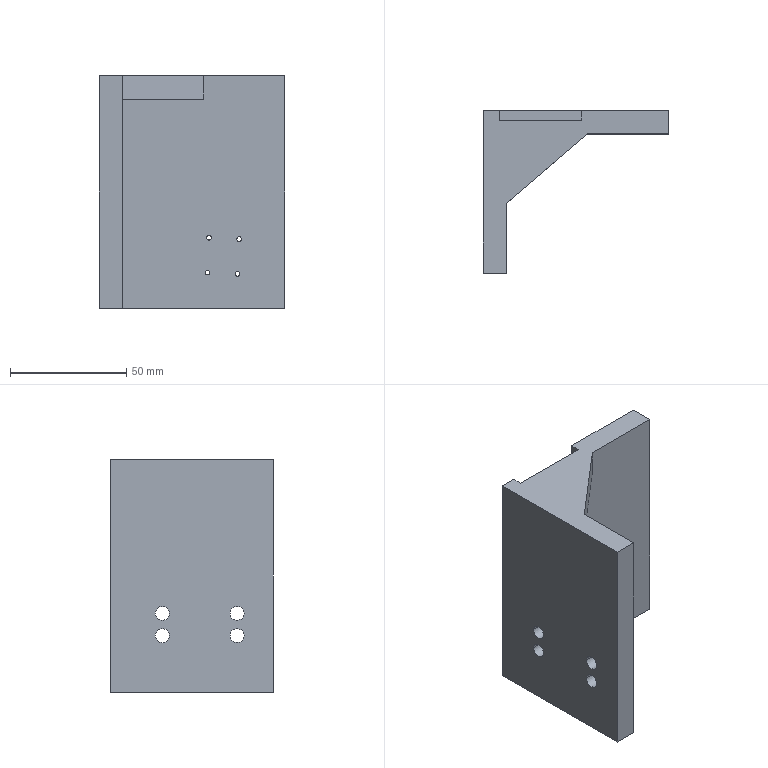Part | SolidWorks | features Cut 3, Extrusion 1, Rib 1 | 1 solid | 30 faces | box 80 x 70 x 100 mm | volume 135093 mm3 | cylinder 16 | plane 14 | commonest cylinder face diameters 2 x8 6 x8
STEP:
#1=CARTESIAN_POINT('',(8.816,32.788,30.301));
#2=VERTEX_POINT('',#1);
#3=CARTESIAN_POINT('',(10.816,32.788,30.301));
#4=VERTEX_POINT('',#3);
#5=CARTESIAN_POINT('',(9.816,32.788,30.301));
#6=DIRECTION('',(0.,-1.,0.));
#7=DIRECTION('',(1.,0.,0.));
#8=AXIS2_PLACEMENT_3D('',#5,#6,#7);
#9=CIRCLE('',#8,1.);
#10=EDGE_CURVE('',#2,#4,#9,.T.);
#11=ORIENTED_EDGE('',*,*,#10,.F.);
#12=CARTESIAN_POINT('',(8.816,22.788,30.301));
#13=VERTEX_POINT('',#12);
#14=CARTESIAN_POINT('',(8.816,37.788,30.301));
#15=DIRECTION('',(0.,-1.,0.));
#16=VECTOR('',#15,1000.);
#17=LINE('',#14,#16);
#18=EDGE_CURVE('',#2,#13,#17,.T.);
#19=ORIENTED_EDGE('',*,*,#18,.T.);
#20=CARTESIAN_POINT('',(10.816,22.788,30.301));
#21=VERTEX_POINT('',#20);
#22=CARTESIAN_POINT('',(9.816,22.788,30.301));
#23=DIRECTION('',(0.,-1.,0.));
#24=DIRECTION('',(1.,0.,0.));
#25=AXIS2_PLACEMENT_3D('',#22,#23,#24);
#26=CIRCLE('',#25,1.);
#27=EDGE_CURVE('',#13,#21,#26,.T.);
#28=ORIENTED_EDGE('',*,*,#27,.T.);
#29=CARTESIAN_POINT('',(10.816,37.788,30.301));
#30=DIRECTION('',(0.,-1.,0.));
#31=VECTOR('',#30,1000.);
#32=LINE('',#29,#31);
#33=EDGE_CURVE('',#4,#21,#32,.T.);
#34=ORIENTED_EDGE('',*,*,#33,.F.);
#35=EDGE_LOOP('',(#11,#19,#28,#34));
#36=FACE_OUTER_BOUND('',#35,.T.);
#37=CARTESIAN_POINT('',(9.816,37.788,30.301));
#38=DIRECTION('',(0.,-1.,0.));
#39=DIRECTION('',(1.,0.,0.));
#40=AXIS2_PLACEMENT_3D('',#37,#38,#39);
#41=CYLINDRICAL_SURFACE('',#40,1.);
#42=ADVANCED_FACE('',(#36),#41,.F.);
#43=CARTESIAN_POINT('',(21.15,32.788,14.748));
#44=VERTEX_POINT('',#43);
#45=CARTESIAN_POINT('',(23.15,32.788,14.748));
#46=VERTEX_POINT('',#45);
#47=CARTESIAN_POINT('',(22.15,32.788,14.748));
#48=DIRECTION('',(0.,-1.,0.));
#49=DIRECTION('',(1.,0.,0.));
#50=AXIS2_PLACEMENT_3D('',#47,#48,#49);
#51=CIRCLE('',#50,1.);
#52=EDGE_CURVE('',#44,#46,#51,.T.);
#53=ORIENTED_EDGE('',*,*,#52,.F.);
#54=CARTESIAN_POINT('',(21.15,22.788,14.748));
#55=VERTEX_POINT('',#54);
#56=CARTESIAN_POINT('',(21.15,37.788,14.748));
#57=DIRECTION('',(0.,-1.,0.));
#58=VECTOR('',#57,1000.);
#59=LINE('',#56,#58);
#60=EDGE_CURVE('',#44,#55,#59,.T.);
#61=ORIENTED_EDGE('',*,*,#60,.T.);
#62=CARTESIAN_POINT('',(23.15,22.788,14.748));
#63=VERTEX_POINT('',#62);
#64=CARTESIAN_POINT('',(22.15,22.788,14.748));
#65=DIRECTION('',(0.,-1.,0.));
#66=DIRECTION('',(1.,0.,0.));
#67=AXIS2_PLACEMENT_3D('',#64,#65,#66);
#68=CIRCLE('',#67,1.);
#69=EDGE_CURVE('',#55,#63,#68,.T.);
#70=ORIENTED_EDGE('',*,*,#69,.T.);
#71=CARTESIAN_POINT('',(23.15,37.788,14.748));
#72=DIRECTION('',(0.,-1.,0.));
#73=VECTOR('',#72,1000.);
#74=LINE('',#71,#73);
#75=EDGE_CURVE('',#46,#63,#74,.T.);
#76=ORIENTED_EDGE('',*,*,#75,.F.);
#77=EDGE_LOOP('',(#53,#61,#70,#76));
#78=FACE_OUTER_BOUND('',#77,.T.);
#79=CARTESIAN_POINT('',(22.15,37.788,14.748));
#80=DIRECTION('',(0.,-1.,0.));
#81=DIRECTION('',(1.,0.,0.));
#82=AXIS2_PLACEMENT_3D('',#79,#80,#81);
#83=CYLINDRICAL_SURFACE('',#82,1.);
#84=ADVANCED_FACE('',(#78),#83,.F.);
#85=CARTESIAN_POINT('',(21.804,32.788,29.734));
#86=VERTEX_POINT('',#85);
#87=CARTESIAN_POINT('',(23.804,32.788,29.734));
#88=VERTEX_POINT('',#87);
#89=CARTESIAN_POINT('',(22.804,32.788,29.734));
#90=DIRECTION('',(0.,-1.,0.));
#91=DIRECTION('',(1.,0.,0.));
#92=AXIS2_PLACEMENT_3D('',#89,#90,#91);
#93=CIRCLE('',#92,1.);
#94=EDGE_CURVE('',#86,#88,#93,.T.);
#95=ORIENTED_EDGE('',*,*,#94,.F.);
#96=CARTESIAN_POINT('',(21.804,22.788,29.734));
#97=VERTEX_POINT('',#96);
#98=CARTESIAN_POINT('',(21.804,37.788,29.734));
#99=DIRECTION('',(0.,-1.,0.));
#100=VECTOR('',#99,1000.);
#101=LINE('',#98,#100);
#102=EDGE_CURVE('',#86,#97,#101,.T.);
#103=ORIENTED_EDGE('',*,*,#102,.T.);
#104=CARTESIAN_POINT('',(23.804,22.788,29.734));
#105=VERTEX_POINT('',#104);
#106=CARTESIAN_POINT('',(22.804,22.788,29.734));
#107=DIRECTION('',(0.,-1.,0.));
#108=DIRECTION('',(1.,0.,0.));
#109=AXIS2_PLACEMENT_3D('',#106,#107,#108);
#110=CIRCLE('',#109,1.);
#111=EDGE_CURVE('',#97,#105,#110,.T.);
#112=ORIENTED_EDGE('',*,*,#111,.T.);
#113=CARTESIAN_POINT('',(23.804,37.788,29.734));
#114=DIRECTION('',(0.,-1.,0.));
#115=VECTOR('',#114,1000.);
#116=LINE('',#113,#115);
#117=EDGE_CURVE('',#88,#105,#116,.T.);
#118=ORIENTED_EDGE('',*,*,#117,.F.);
#119=EDGE_LOOP('',(#95,#103,#112,#118));
#120=FACE_OUTER_BOUND('',#119,.T.);
#121=CARTESIAN_POINT('',(22.804,37.788,29.734));
#122=DIRECTION('',(0.,-1.,0.));
#123=DIRECTION('',(1.,0.,0.));
#124=AXIS2_PLACEMENT_3D('',#121,#122,#123);
#125=CYLINDRICAL_SURFACE('',#124,1.);
#126=ADVANCED_FACE('',(#120),#125,.F.);
#127=CARTESIAN_POINT('',(8.162,32.788,15.315));
#128=VERTEX_POINT('',#127);
#129=CARTESIAN_POINT('',(10.162,32.788,15.315));
#130=VERTEX_POINT('',#129);
#131=CARTESIAN_POINT('',(9.162,32.788,15.315));
#132=DIRECTION('',(0.,-1.,0.));
#133=DIRECTION('',(1.,0.,0.));
#134=AXIS2_PLACEMENT_3D('',#131,#132,#133);
#135=CIRCLE('',#134,1.);
#136=EDGE_CURVE('',#128,#130,#135,.T.);
#137=ORIENTED_EDGE('',*,*,#136,.F.);
#138=CARTESIAN_POINT('',(8.162,22.788,15.315));
#139=VERTEX_POINT('',#138);
#140=CARTESIAN_POINT('',(8.162,37.788,15.315));
#141=DIRECTION('',(0.,-1.,0.));
#142=VECTOR('',#141,1000.);
#143=LINE('',#140,#142);
#144=EDGE_CURVE('',#128,#139,#143,.T.);
#145=ORIENTED_EDGE('',*,*,#144,.T.);
#146=CARTESIAN_POINT('',(10.162,22.788,15.315));
#147=VERTEX_POINT('',#146);
#148=CARTESIAN_POINT('',(9.162,22.788,15.315));
#149=DIRECTION('',(0.,-1.,0.));
#150=DIRECTION('',(1.,0.,0.));
#151=AXIS2_PLACEMENT_3D('',#148,#149,#150);
#152=CIRCLE('',#151,1.);
#153=EDGE_CURVE('',#139,#147,#152,.T.);
#154=ORIENTED_EDGE('',*,*,#153,.T.);
#155=CARTESIAN_POINT('',(10.162,37.788,15.315));
#156=DIRECTION('',(0.,-1.,0.));
#157=VECTOR('',#156,1000.);
#158=LINE('',#155,#157);
#159=EDGE_CURVE('',#130,#147,#158,.T.);
#160=ORIENTED_EDGE('',*,*,#159,.F.);
#161=EDGE_LOOP('',(#137,#145,#154,#160));
#162=FACE_OUTER_BOUND('',#161,.T.);
#163=CARTESIAN_POINT('',(9.162,37.788,15.315));
#164=DIRECTION('',(0.,-1.,0.));
#165=DIRECTION('',(1.,0.,0.));
#166=AXIS2_PLACEMENT_3D('',#163,#164,#165);
#167=CYLINDRICAL_SURFACE('',#166,1.);
#168=ADVANCED_FACE('',(#162),#167,.F.);
#169=CARTESIAN_POINT('',(-37.5,-18.605,24.355));
#170=VERTEX_POINT('',#169);
#171=CARTESIAN_POINT('',(-37.5,-24.605,24.355));
#172=VERTEX_POINT('',#171);
#173=CARTESIAN_POINT('',(-37.5,-21.605,24.355));
#174=DIRECTION('',(-1.,0.,0.));
#175=DIRECTION('',(0.,0.,-1.));
#176=AXIS2_PLACEMENT_3D('',#173,#174,#175);
#177=CIRCLE('',#176,3.);
#178=EDGE_CURVE('',#170,#172,#177,.T.);
#179=ORIENTED_EDGE('',*,*,#178,.T.);
#180=CARTESIAN_POINT('',(-27.5,-24.605,24.355));
#181=VERTEX_POINT('',#180);
#182=CARTESIAN_POINT('',(-45.985,-24.605,24.355));
#183=DIRECTION('',(1.,0.,0.));
#184=VECTOR('',#183,1000.);
#185=LINE('',#182,#184);
#186=EDGE_CURVE('',#172,#181,#185,.T.);
#187=ORIENTED_EDGE('',*,*,#186,.T.);
#188=CARTESIAN_POINT('',(-27.5,-18.605,24.355));
#189=VERTEX_POINT('',#188);
#190=CARTESIAN_POINT('',(-27.5,-21.605,24.355));
#191=DIRECTION('',(1.,0.,0.));
#192=DIRECTION('',(0.,1.,0.));
#193=AXIS2_PLACEMENT_3D('',#190,#191,#192);
#194=CIRCLE('',#193,3.);
#195=EDGE_CURVE('',#181,#189,#194,.T.);
#196=ORIENTED_EDGE('',*,*,#195,.T.);
#197=CARTESIAN_POINT('',(-45.985,-18.605,24.355));
#198=DIRECTION('',(1.,0.,0.));
#199=VECTOR('',#198,1000.);
#200=LINE('',#197,#199);
#201=EDGE_CURVE('',#170,#189,#200,.T.);
#202=ORIENTED_EDGE('',*,*,#201,.F.);
#203=EDGE_LOOP('',(#179,#187,#196,#202));
#204=FACE_OUTER_BOUND('',#203,.T.);
#205=CARTESIAN_POINT('',(-45.985,-21.605,24.355));
#206=DIRECTION('',(1.,0.,0.));
#207=DIRECTION('',(0.,1.,0.));
#208=AXIS2_PLACEMENT_3D('',#205,#206,#207);
#209=CYLINDRICAL_SURFACE('',#208,3.);
#210=ADVANCED_FACE('',(#204),#209,.F.);
#211=CARTESIAN_POINT('',(-37.5,13.563,24.355));
#212=VERTEX_POINT('',#211);
#213=CARTESIAN_POINT('',(-37.5,7.563,24.355));
#214=VERTEX_POINT('',#213);
#215=CARTESIAN_POINT('',(-37.5,10.563,24.355));
#216=DIRECTION('',(-1.,0.,0.));
#217=DIRECTION('',(0.,0.,-1.));
#218=AXIS2_PLACEMENT_3D('',#215,#216,#217);
#219=CIRCLE('',#218,3.);
#220=EDGE_CURVE('',#212,#214,#219,.T.);
#221=ORIENTED_EDGE('',*,*,#220,.T.);
#222=CARTESIAN_POINT('',(-27.5,7.563,24.355));
#223=VERTEX_POINT('',#222);
#224=CARTESIAN_POINT('',(-45.985,7.563,24.355));
#225=DIRECTION('',(1.,0.,0.));
#226=VECTOR('',#225,1000.);
#227=LINE('',#224,#226);
#228=EDGE_CURVE('',#214,#223,#227,.T.);
#229=ORIENTED_EDGE('',*,*,#228,.T.);
#230=CARTESIAN_POINT('',(-27.5,13.563,24.355));
#231=VERTEX_POINT('',#230);
#232=CARTESIAN_POINT('',(-27.5,10.563,24.355));
#233=DIRECTION('',(1.,0.,0.));
#234=DIRECTION('',(0.,1.,0.));
#235=AXIS2_PLACEMENT_3D('',#232,#233,#234);
#236=CIRCLE('',#235,3.);
#237=EDGE_CURVE('',#223,#231,#236,.T.);
#238=ORIENTED_EDGE('',*,*,#237,.T.);
#239=CARTESIAN_POINT('',(-45.985,13.563,24.355));
#240=DIRECTION('',(1.,0.,0.));
#241=VECTOR('',#240,1000.);
#242=LINE('',#239,#241);
#243=EDGE_CURVE('',#212,#231,#242,.T.);
#244=ORIENTED_EDGE('',*,*,#243,.F.);
#245=EDGE_LOOP('',(#221,#229,#238,#244));
#246=FACE_OUTER_BOUND('',#245,.T.);
#247=CARTESIAN_POINT('',(-45.985,10.563,24.355));
#248=DIRECTION('',(1.,0.,0.));
#249=DIRECTION('',(0.,1.,0.));
#250=AXIS2_PLACEMENT_3D('',#247,#248,#249);
#251=CYLINDRICAL_SURFACE('',#250,3.);
#252=ADVANCED_FACE('',(#246),#251,.F.);
#253=CARTESIAN_POINT('',(-37.5,13.563,33.892));
#254=VERTEX_POINT('',#253);
#255=CARTESIAN_POINT('',(-37.5,7.563,33.892));
#256=VERTEX_POINT('',#255);
#257=CARTESIAN_POINT('',(-37.5,10.563,33.892));
#258=DIRECTION('',(-1.,0.,0.));
#259=DIRECTION('',(0.,0.,-1.));
#260=AXIS2_PLACEMENT_3D('',#257,#258,#259);
#261=CIRCLE('',#260,3.);
#262=EDGE_CURVE('',#254,#256,#261,.T.);
#263=ORIENTED_EDGE('',*,*,#262,.T.);
#264=CARTESIAN_POINT('',(-27.5,7.563,33.892));
#265=VERTEX_POINT('',#264);
#266=CARTESIAN_POINT('',(-45.985,7.563,33.892));
#267=DIRECTION('',(1.,0.,0.));
#268=VECTOR('',#267,1000.);
#269=LINE('',#266,#268);
#270=EDGE_CURVE('',#256,#265,#269,.T.);
#271=ORIENTED_EDGE('',*,*,#270,.T.);
#272=CARTESIAN_POINT('',(-27.5,13.563,33.892));
#273=VERTEX_POINT('',#272);
#274=CARTESIAN_POINT('',(-27.5,10.563,33.892));
#275=DIRECTION('',(1.,0.,0.));
#276=DIRECTION('',(0.,1.,0.));
#277=AXIS2_PLACEMENT_3D('',#274,#275,#276);
#278=CIRCLE('',#277,3.);
#279=EDGE_CURVE('',#265,#273,#278,.T.);
#280=ORIENTED_EDGE('',*,*,#279,.T.);
#281=CARTESIAN_POINT('',(-45.985,13.563,33.892));
#282=DIRECTION('',(1.,0.,0.));
#283=VECTOR('',#282,1000.);
#284=LINE('',#281,#283);
#285=EDGE_CURVE('',#254,#273,#284,.T.);
#286=ORIENTED_EDGE('',*,*,#285,.F.);
#287=EDGE_LOOP('',(#263,#271,#280,#286));
#288=FACE_OUTER_BOUND('',#287,.T.);
#289=CARTESIAN_POINT('',(-45.985,10.563,33.892));
#290=DIRECTION('',(1.,0.,0.));
#291=DIRECTION('',(0.,1.,0.));
#292=AXIS2_PLACEMENT_3D('',#289,#290,#291);
#293=CYLINDRICAL_SURFACE('',#292,3.);
#294=ADVANCED_FACE('',(#288),#293,.F.);
#295=CARTESIAN_POINT('',(-37.5,-18.605,33.892));
#296=VERTEX_POINT('',#295);
#297=CARTESIAN_POINT('',(-37.5,-24.605,33.892));
#298=VERTEX_POINT('',#297);
#299=CARTESIAN_POINT('',(-37.5,-21.605,33.892));
#300=DIRECTION('',(-1.,0.,0.));
#301=DIRECTION('',(0.,0.,-1.));
#302=AXIS2_PLACEMENT_3D('',#299,#300,#301);
#303=CIRCLE('',#302,3.);
#304=EDGE_CURVE('',#296,#298,#303,.T.);
#305=ORIENTED_EDGE('',*,*,#304,.T.);
#306=CARTESIAN_POINT('',(-27.5,-24.605,33.892));
#307=VERTEX_POINT('',#306);
#308=CARTESIAN_POINT('',(-45.985,-24.605,33.892));
#309=DIRECTION('',(1.,0.,0.));
#310=VECTOR('',#309,1000.);
#311=LINE('',#308,#310);
#312=EDGE_CURVE('',#298,#307,#311,.T.);
#313=ORIENTED_EDGE('',*,*,#312,.T.);
#314=CARTESIAN_POINT('',(-27.5,-18.605,33.892));
#315=VERTEX_POINT('',#314);
#316=CARTESIAN_POINT('',(-27.5,-21.605,33.892));
#317=DIRECTION('',(1.,0.,0.));
#318=DIRECTION('',(0.,1.,0.));
#319=AXIS2_PLACEMENT_3D('',#316,#317,#318);
#320=CIRCLE('',#319,3.);
#321=EDGE_CURVE('',#307,#315,#320,.T.);
#322=ORIENTED_EDGE('',*,*,#321,.T.);
#323=CARTESIAN_POINT('',(-45.985,-18.605,33.892));
#324=DIRECTION('',(1.,0.,0.));
#325=VECTOR('',#324,1000.);
#326=LINE('',#323,#325);
#327=EDGE_CURVE('',#296,#315,#326,.T.);
#328=ORIENTED_EDGE('',*,*,#327,.F.);
#329=EDGE_LOOP('',(#305,#313,#322,#328));
#330=FACE_OUTER_BOUND('',#329,.T.);
#331=CARTESIAN_POINT('',(-45.985,-21.605,33.892));
#332=DIRECTION('',(1.,0.,0.));
#333=DIRECTION('',(0.,1.,0.));
#334=AXIS2_PLACEMENT_3D('',#331,#332,#333);
#335=CYLINDRICAL_SURFACE('',#334,3.);
#336=ADVANCED_FACE('',(#330),#335,.F.);
#337=ORIENTED_EDGE('',*,*,#178,.F.);
#338=CARTESIAN_POINT('',(-37.5,-21.605,24.355));
#339=DIRECTION('',(-1.,0.,0.));
#340=DIRECTION('',(0.,0.,-1.));
#341=AXIS2_PLACEMENT_3D('',#338,#339,#340);
#342=CIRCLE('',#341,3.);
#343=EDGE_CURVE('',#172,#170,#342,.T.);
#344=ORIENTED_EDGE('',*,*,#343,.F.);
#345=EDGE_LOOP('',(#337,#344));
#346=FACE_BOUND('',#345,.T.);
#347=ORIENTED_EDGE('',*,*,#220,.F.);
#348=CARTESIAN_POINT('',(-37.5,10.563,24.355));
#349=DIRECTION('',(-1.,0.,0.));
#350=DIRECTION('',(0.,0.,-1.));
#351=AXIS2_PLACEMENT_3D('',#348,#349,#350);
#352=CIRCLE('',#351,3.);
#353=EDGE_CURVE('',#214,#212,#352,.T.);
#354=ORIENTED_EDGE('',*,*,#353,.F.);
#355=EDGE_LOOP('',(#347,#354));
#356=FACE_BOUND('',#355,.T.);
#357=ORIENTED_EDGE('',*,*,#262,.F.);
#358=CARTESIAN_POINT('',(-37.5,10.563,33.892));
#359=DIRECTION('',(-1.,0.,0.));
#360=DIRECTION('',(0.,0.,-1.));
#361=AXIS2_PLACEMENT_3D('',#358,#359,#360);
#362=CIRCLE('',#361,3.);
#363=EDGE_CURVE('',#256,#254,#362,.T.);
#364=ORIENTED_EDGE('',*,*,#363,.F.);
#365=EDGE_LOOP('',(#357,#364));
#366=FACE_BOUND('',#365,.T.);
#367=ORIENTED_EDGE('',*,*,#304,.F.);
#368=CARTESIAN_POINT('',(-37.5,-21.605,33.892));
#369=DIRECTION('',(-1.,0.,0.));
#370=DIRECTION('',(0.,0.,-1.));
#371=AXIS2_PLACEMENT_3D('',#368,#369,#370);
#372=CIRCLE('',#371,3.);
#373=EDGE_CURVE('',#298,#296,#372,.T.);
#374=ORIENTED_EDGE('',*,*,#373,.F.);
#375=EDGE_LOOP('',(#367,#374));
#376=FACE_BOUND('',#375,.T.);
#377=CARTESIAN_POINT('',(-37.5,-37.212,100.));
#378=VERTEX_POINT('',#377);
#379=CARTESIAN_POINT('',(-37.5,-37.212,0.));
#380=VERTEX_POINT('',#379);
#381=CARTESIAN_POINT('',(-37.5,-37.212,100.));
#382=DIRECTION('',(0.,0.,-1.));
#383=VECTOR('',#382,1000.);
#384=LINE('',#381,#383);
#385=EDGE_CURVE('',#378,#380,#384,.T.);
#386=ORIENTED_EDGE('',*,*,#385,.F.);
#387=CARTESIAN_POINT('',(-37.5,32.788,100.));
#388=VERTEX_POINT('',#387);
#389=CARTESIAN_POINT('',(-37.5,-37.212,100.));
#390=DIRECTION('',(0.,-1.,0.));
#391=VECTOR('',#390,1000.);
#392=LINE('',#389,#391);
#393=EDGE_CURVE('',#388,#378,#392,.T.);
#394=ORIENTED_EDGE('',*,*,#393,.F.);
#395=CARTESIAN_POINT('',(-37.5,32.788,0.));
#396=VERTEX_POINT('',#395);
#397=CARTESIAN_POINT('',(-37.5,32.788,100.));
#398=DIRECTION('',(0.,0.,-1.));
#399=VECTOR('',#398,1000.);
#400=LINE('',#397,#399);
#401=EDGE_CURVE('',#388,#396,#400,.T.);
#402=ORIENTED_EDGE('',*,*,#401,.T.);
#403=CARTESIAN_POINT('',(-37.5,-37.212,0.));
#404=DIRECTION('',(0.,-1.,0.));
#405=VECTOR('',#404,1000.);
#406=LINE('',#403,#405);
#407=EDGE_CURVE('',#396,#380,#406,.T.);
#408=ORIENTED_EDGE('',*,*,#407,.T.);
#409=EDGE_LOOP('',(#386,#394,#402,#408));
#410=FACE_OUTER_BOUND('',#409,.T.);
#411=CARTESIAN_POINT('',(-37.5,-37.212,100.));
#412=DIRECTION('',(1.,0.,0.));
#413=DIRECTION('',(0.,0.,-1.));
#414=AXIS2_PLACEMENT_3D('',#411,#412,#413);
#415=PLANE('',#414);
#416=ADVANCED_FACE('',(#346,#356,#366,#376,#410),#415,.F.);
#417=CARTESIAN_POINT('',(-27.5,-37.212,0.));
#418=VERTEX_POINT('',#417);
#419=CARTESIAN_POINT('',(-27.5,-37.212,0.));
#420=DIRECTION('',(1.,0.,0.));
#421=VECTOR('',#420,1000.);
#422=LINE('',#419,#421);
#423=EDGE_CURVE('',#380,#418,#422,.T.);
#424=ORIENTED_EDGE('',*,*,#423,.T.);
#425=CARTESIAN_POINT('',(-27.5,-37.212,100.));
#426=VERTEX_POINT('',#425);
#427=CARTESIAN_POINT('',(-27.5,-37.212,100.));
#428=DIRECTION('',(0.,0.,-1.));
#429=VECTOR('',#428,1000.);
#430=LINE('',#427,#429);
#431=EDGE_CURVE('',#426,#418,#430,.T.);
#432=ORIENTED_EDGE('',*,*,#431,.F.);
#433=CARTESIAN_POINT('',(-27.5,-37.212,100.));
#434=DIRECTION('',(1.,0.,0.));
#435=VECTOR('',#434,1000.);
#436=LINE('',#433,#435);
#437=EDGE_CURVE('',#378,#426,#436,.T.);
#438=ORIENTED_EDGE('',*,*,#437,.F.);
#439=ORIENTED_EDGE('',*,*,#385,.T.);
#440=EDGE_LOOP('',(#424,#432,#438,#439));
#441=FACE_OUTER_BOUND('',#440,.T.);
#442=CARTESIAN_POINT('',(-27.5,-37.212,100.));
#443=DIRECTION('',(0.,1.,0.));
#444=DIRECTION('',(0.,0.,1.));
#445=AXIS2_PLACEMENT_3D('',#442,#443,#444);
#446=PLANE('',#445);
#447=ADVANCED_FACE('',(#441),#446,.F.);
#448=CARTESIAN_POINT('',(-27.5,-21.605,24.355));
#449=DIRECTION('',(1.,0.,0.));
#450=DIRECTION('',(0.,1.,0.));
#451=AXIS2_PLACEMENT_3D('',#448,#449,#450);
#452=CIRCLE('',#451,3.);
#453=EDGE_CURVE('',#189,#181,#452,.T.);
#454=ORIENTED_EDGE('',*,*,#453,.F.);
#455=ORIENTED_EDGE('',*,*,#195,.F.);
#456=EDGE_LOOP('',(#454,#455));
#457=FACE_BOUND('',#456,.T.);
#458=CARTESIAN_POINT('',(-27.5,10.563,24.355));
#459=DIRECTION('',(1.,0.,0.));
#460=DIRECTION('',(0.,1.,0.));
#461=AXIS2_PLACEMENT_3D('',#458,#459,#460);
#462=CIRCLE('',#461,3.);
#463=EDGE_CURVE('',#231,#223,#462,.T.);
#464=ORIENTED_EDGE('',*,*,#463,.F.);
#465=ORIENTED_EDGE('',*,*,#237,.F.);
#466=EDGE_LOOP('',(#464,#465));
#467=FACE_BOUND('',#466,.T.);
#468=CARTESIAN_POINT('',(-27.5,10.563,33.892));
#469=DIRECTION('',(1.,0.,0.));
#470=DIRECTION('',(0.,1.,0.));
#471=AXIS2_PLACEMENT_3D('',#468,#469,#470);
#472=CIRCLE('',#471,3.);
#473=EDGE_CURVE('',#273,#265,#472,.T.);
#474=ORIENTED_EDGE('',*,*,#473,.F.);
#475=ORIENTED_EDGE('',*,*,#279,.F.);
#476=EDGE_LOOP('',(#474,#475));
#477=FACE_BOUND('',#476,.T.);
#478=CARTESIAN_POINT('',(-27.5,-21.605,33.892));
#479=DIRECTION('',(1.,0.,0.));
#480=DIRECTION('',(0.,1.,0.));
#481=AXIS2_PLACEMENT_3D('',#478,#479,#480);
#482=CIRCLE('',#481,3.);
#483=EDGE_CURVE('',#315,#307,#482,.T.);
#484=ORIENTED_EDGE('',*,*,#483,.F.);
#485=ORIENTED_EDGE('',*,*,#321,.F.);
#486=EDGE_LOOP('',(#484,#485));
#487=FACE_BOUND('',#486,.T.);
#488=CARTESIAN_POINT('',(-27.5,-7.212,90.));
#489=VERTEX_POINT('',#488);
#490=CARTESIAN_POINT('',(-27.5,22.788,90.));
#491=VERTEX_POINT('',#490);
#492=CARTESIAN_POINT('',(-27.5,22.788,90.));
#493=DIRECTION('',(0.,1.,0.));
#494=VECTOR('',#493,1000.);
#495=LINE('',#492,#494);
#496=EDGE_CURVE('',#489,#491,#495,.T.);
#497=ORIENTED_EDGE('',*,*,#496,.F.);
#498=CARTESIAN_POINT('',(-27.5,-7.212,100.));
#499=VERTEX_POINT('',#498);
#500=CARTESIAN_POINT('',(-27.5,-7.212,100.));
#501=DIRECTION('',(0.,0.,1.));
#502=VECTOR('',#501,1000.);
#503=LINE('',#500,#502);
#504=EDGE_CURVE('',#489,#499,#503,.T.);
#505=ORIENTED_EDGE('',*,*,#504,.T.);
#506=CARTESIAN_POINT('',(-27.5,22.788,100.));
#507=DIRECTION('',(0.,1.,0.));
#508=VECTOR('',#507,1000.);
#509=LINE('',#506,#508);
#510=EDGE_CURVE('',#426,#499,#509,.T.);
#511=ORIENTED_EDGE('',*,*,#510,.F.);
#512=ORIENTED_EDGE('',*,*,#431,.T.);
#513=CARTESIAN_POINT('',(-27.5,22.788,0.));
#514=VERTEX_POINT('',#513);
#515=CARTESIAN_POINT('',(-27.5,22.788,0.));
#516=DIRECTION('',(0.,1.,0.));
#517=VECTOR('',#516,1000.);
#518=LINE('',#515,#517);
#519=EDGE_CURVE('',#418,#514,#518,.T.);
#520=ORIENTED_EDGE('',*,*,#519,.T.);
#521=CARTESIAN_POINT('',(-27.5,22.788,100.));
#522=DIRECTION('',(0.,0.,-1.));
#523=VECTOR('',#522,1000.);
#524=LINE('',#521,#523);
#525=EDGE_CURVE('',#491,#514,#524,.T.);
#526=ORIENTED_EDGE('',*,*,#525,.F.);
#527=EDGE_LOOP('',(#497,#505,#511,#512,#520,#526));
#528=FACE_OUTER_BOUND('',#527,.T.);
#529=CARTESIAN_POINT('',(-27.5,22.788,100.));
#530=DIRECTION('',(-1.,0.,0.));
#531=DIRECTION('',(0.,-1.,0.));
#532=AXIS2_PLACEMENT_3D('',#529,#530,#531);
#533=PLANE('',#532);
#534=ADVANCED_FACE('',(#457,#467,#477,#487,#528),#533,.F.);
#535=CARTESIAN_POINT('',(9.816,22.788,30.301));
#536=DIRECTION('',(0.,-1.,0.));
#537=DIRECTION('',(1.,0.,0.));
#538=AXIS2_PLACEMENT_3D('',#535,#536,#537);
#539=CIRCLE('',#538,1.);
#540=EDGE_CURVE('',#21,#13,#539,.T.);
#541=ORIENTED_EDGE('',*,*,#540,.F.);
#542=ORIENTED_EDGE('',*,*,#27,.F.);
#543=EDGE_LOOP('',(#541,#542));
#544=FACE_BOUND('',#543,.T.);
#545=CARTESIAN_POINT('',(22.15,22.788,14.748));
#546=DIRECTION('',(0.,-1.,0.));
#547=DIRECTION('',(1.,0.,0.));
#548=AXIS2_PLACEMENT_3D('',#545,#546,#547);
#549=CIRCLE('',#548,1.);
#550=EDGE_CURVE('',#63,#55,#549,.T.);
#551=ORIENTED_EDGE('',*,*,#550,.F.);
#552=ORIENTED_EDGE('',*,*,#69,.F.);
#553=EDGE_LOOP('',(#551,#552));
#554=FACE_BOUND('',#553,.T.);
#555=CARTESIAN_POINT('',(22.804,22.788,29.734));
#556=DIRECTION('',(0.,-1.,0.));
#557=DIRECTION('',(1.,0.,0.));
#558=AXIS2_PLACEMENT_3D('',#555,#556,#557);
#559=CIRCLE('',#558,1.);
#560=EDGE_CURVE('',#105,#97,#559,.T.);
#561=ORIENTED_EDGE('',*,*,#560,.F.);
#562=ORIENTED_EDGE('',*,*,#111,.F.);
#563=EDGE_LOOP('',(#561,#562));
#564=FACE_BOUND('',#563,.T.);
#565=CARTESIAN_POINT('',(9.162,22.788,15.315));
#566=DIRECTION('',(0.,-1.,0.));
#567=DIRECTION('',(1.,0.,0.));
#568=AXIS2_PLACEMENT_3D('',#565,#566,#567);
#569=CIRCLE('',#568,1.);
#570=EDGE_CURVE('',#147,#139,#569,.T.);
#571=ORIENTED_EDGE('',*,*,#570,.F.);
#572=ORIENTED_EDGE('',*,*,#153,.F.);
#573=EDGE_LOOP('',(#571,#572));
#574=FACE_BOUND('',#573,.T.);
#575=CARTESIAN_POINT('',(7.5,22.788,100.));
#576=VERTEX_POINT('',#575);
#577=CARTESIAN_POINT('',(42.5,22.788,100.));
#578=VERTEX_POINT('',#577);
#579=CARTESIAN_POINT('',(42.5,22.788,100.));
#580=DIRECTION('',(1.,0.,0.));
#581=VECTOR('',#580,1000.);
#582=LINE('',#579,#581);
#583=EDGE_CURVE('',#576,#578,#582,.T.);
#584=ORIENTED_EDGE('',*,*,#583,.F.);
#585=CARTESIAN_POINT('',(7.5,22.788,90.));
#586=VERTEX_POINT('',#585);
#587=CARTESIAN_POINT('',(7.5,22.788,100.));
#588=DIRECTION('',(0.,0.,-1.));
#589=VECTOR('',#588,1000.);
#590=LINE('',#587,#589);
#591=EDGE_CURVE('',#576,#586,#590,.T.);
#592=ORIENTED_EDGE('',*,*,#591,.T.);
#593=CARTESIAN_POINT('',(42.5,22.788,90.));
#594=DIRECTION('',(1.,0.,0.));
#595=VECTOR('',#594,1000.);
#596=LINE('',#593,#595);
#597=EDGE_CURVE('',#491,#586,#596,.T.);
#598=ORIENTED_EDGE('',*,*,#597,.F.);
#599=ORIENTED_EDGE('',*,*,#525,.T.);
#600=CARTESIAN_POINT('',(42.5,22.788,0.));
#601=VERTEX_POINT('',#600);
#602=CARTESIAN_POINT('',(42.5,22.788,0.));
#603=DIRECTION('',(1.,0.,0.));
#604=VECTOR('',#603,1000.);
#605=LINE('',#602,#604);
#606=EDGE_CURVE('',#514,#601,#605,.T.);
#607=ORIENTED_EDGE('',*,*,#606,.T.);
#608=CARTESIAN_POINT('',(42.5,22.788,100.));
#609=DIRECTION('',(0.,0.,-1.));
#610=VECTOR('',#609,1000.);
#611=LINE('',#608,#610);
#612=EDGE_CURVE('',#578,#601,#611,.T.);
#613=ORIENTED_EDGE('',*,*,#612,.F.);
#614=EDGE_LOOP('',(#584,#592,#598,#599,#607,#613));
#615=FACE_OUTER_BOUND('',#614,.T.);
#616=CARTESIAN_POINT('',(42.5,22.788,100.));
#617=DIRECTION('',(0.,1.,0.));
#618=DIRECTION('',(-1.,0.,0.));
#619=AXIS2_PLACEMENT_3D('',#616,#617,#618);
#620=PLANE('',#619);
#621=ADVANCED_FACE('',(#544,#554,#564,#574,#615),#620,.F.);
#622=CARTESIAN_POINT('',(42.5,32.788,0.));
#623=VERTEX_POINT('',#622);
#624=CARTESIAN_POINT('',(42.5,32.788,0.));
#625=DIRECTION('',(0.,1.,0.));
#626=VECTOR('',#625,1000.);
#627=LINE('',#624,#626);
#628=EDGE_CURVE('',#601,#623,#627,.T.);
#629=ORIENTED_EDGE('',*,*,#628,.T.);
#630=CARTESIAN_POINT('',(42.5,32.788,100.));
#631=VERTEX_POINT('',#630);
#632=CARTESIAN_POINT('',(42.5,32.788,100.));
#633=DIRECTION('',(0.,0.,-1.));
#634=VECTOR('',#633,1000.);
#635=LINE('',#632,#634);
#636=EDGE_CURVE('',#631,#623,#635,.T.);
#637=ORIENTED_EDGE('',*,*,#636,.F.);
#638=CARTESIAN_POINT('',(42.5,32.788,100.));
#639=DIRECTION('',(0.,1.,0.));
#640=VECTOR('',#639,1000.);
#641=LINE('',#638,#640);
#642=EDGE_CURVE('',#578,#631,#641,.T.);
#643=ORIENTED_EDGE('',*,*,#642,.F.);
#644=ORIENTED_EDGE('',*,*,#612,.T.);
#645=EDGE_LOOP('',(#629,#637,#643,#644));
#646=FACE_OUTER_BOUND('',#645,.T.);
#647=CARTESIAN_POINT('',(42.5,32.788,100.));
#648=DIRECTION('',(-1.,0.,0.));
#649=DIRECTION('',(0.,0.,1.));
#650=AXIS2_PLACEMENT_3D('',#647,#648,#649);
#651=PLANE('',#650);
#652=ADVANCED_FACE('',(#646),#651,.F.);
#653=CARTESIAN_POINT('',(9.816,32.788,30.301));
#654=DIRECTION('',(0.,-1.,0.));
#655=DIRECTION('',(1.,0.,0.));
#656=AXIS2_PLACEMENT_3D('',#653,#654,#655);
#657=CIRCLE('',#656,1.);
#658=EDGE_CURVE('',#4,#2,#657,.T.);
#659=ORIENTED_EDGE('',*,*,#658,.T.);
#660=ORIENTED_EDGE('',*,*,#10,.T.);
#661=EDGE_LOOP('',(#659,#660));
#662=FACE_BOUND('',#661,.T.);
#663=CARTESIAN_POINT('',(22.15,32.788,14.748));
#664=DIRECTION('',(0.,-1.,0.));
#665=DIRECTION('',(1.,0.,0.));
#666=AXIS2_PLACEMENT_3D('',#663,#664,#665);
#667=CIRCLE('',#666,1.);
#668=EDGE_CURVE('',#46,#44,#667,.T.);
#669=ORIENTED_EDGE('',*,*,#668,.T.);
#670=ORIENTED_EDGE('',*,*,#52,.T.);
#671=EDGE_LOOP('',(#669,#670));
#672=FACE_BOUND('',#671,.T.);
#673=CARTESIAN_POINT('',(22.804,32.788,29.734));
#674=DIRECTION('',(0.,-1.,0.));
#675=DIRECTION('',(1.,0.,0.));
#676=AXIS2_PLACEMENT_3D('',#673,#674,#675);
#677=CIRCLE('',#676,1.);
#678=EDGE_CURVE('',#88,#86,#677,.T.);
#679=ORIENTED_EDGE('',*,*,#678,.T.);
#680=ORIENTED_EDGE('',*,*,#94,.T.);
#681=EDGE_LOOP('',(#679,#680));
#682=FACE_BOUND('',#681,.T.);
#683=CARTESIAN_POINT('',(9.162,32.788,15.315));
#684=DIRECTION('',(0.,-1.,0.));
#685=DIRECTION('',(1.,0.,0.));
#686=AXIS2_PLACEMENT_3D('',#683,#684,#685);
#687=CIRCLE('',#686,1.);
#688=EDGE_CURVE('',#130,#128,#687,.T.);
#689=ORIENTED_EDGE('',*,*,#688,.T.);
#690=ORIENTED_EDGE('',*,*,#136,.T.);
#691=EDGE_LOOP('',(#689,#690));
#692=FACE_BOUND('',#691,.T.);
#693=CARTESIAN_POINT('',(4.86,32.788,40.));
#694=VERTEX_POINT('',#693);
#695=CARTESIAN_POINT('',(4.86,32.788,100.));
#696=VERTEX_POINT('',#695);
#697=CARTESIAN_POINT('',(4.86,32.788,40.));
#698=DIRECTION('',(0.,0.,1.));
#699=VECTOR('',#698,1000.);
#700=LINE('',#697,#699);
#701=EDGE_CURVE('',#694,#696,#700,.T.);
#702=ORIENTED_EDGE('',*,*,#701,.T.);
#703=CARTESIAN_POINT('',(-37.5,32.788,100.));
#704=DIRECTION('',(-1.,0.,0.));
#705=VECTOR('',#704,1000.);
#706=LINE('',#703,#705);
#707=EDGE_CURVE('',#631,#696,#706,.T.);
#708=ORIENTED_EDGE('',*,*,#707,.F.);
#709=ORIENTED_EDGE('',*,*,#636,.T.);
#710=CARTESIAN_POINT('',(-37.5,32.788,0.));
#711=DIRECTION('',(-1.,0.,0.));
#712=VECTOR('',#711,1000.);
#713=LINE('',#710,#712);
#714=EDGE_CURVE('',#623,#396,#713,.T.);
#715=ORIENTED_EDGE('',*,*,#714,.T.);
#716=ORIENTED_EDGE('',*,*,#401,.F.);
#717=CARTESIAN_POINT('',(-30.458,32.788,100.));
#718=VERTEX_POINT('',#717);
#719=CARTESIAN_POINT('',(-37.5,32.788,100.));
#720=DIRECTION('',(-1.,0.,0.));
#721=VECTOR('',#720,1000.);
#722=LINE('',#719,#721);
#723=EDGE_CURVE('',#718,#388,#722,.T.);
#724=ORIENTED_EDGE('',*,*,#723,.F.);
#725=CARTESIAN_POINT('',(-30.458,32.788,40.));
#726=VERTEX_POINT('',#725);
#727=CARTESIAN_POINT('',(-30.458,32.788,40.));
#728=DIRECTION('',(0.,0.,1.));
#729=VECTOR('',#728,1000.);
#730=LINE('',#727,#729);
#731=EDGE_CURVE('',#726,#718,#730,.T.);
#732=ORIENTED_EDGE('',*,*,#731,.F.);
#733=CARTESIAN_POINT('',(4.86,32.788,40.));
#734=DIRECTION('',(-1.,0.,0.));
#735=VECTOR('',#734,1000.);
#736=LINE('',#733,#735);
#737=EDGE_CURVE('',#694,#726,#736,.T.);
#738=ORIENTED_EDGE('',*,*,#737,.F.);
#739=EDGE_LOOP('',(#702,#708,#709,#715,#716,#724,#732,#738));
#740=FACE_OUTER_BOUND('',#739,.T.);
#741=CARTESIAN_POINT('',(-37.5,32.788,100.));
#742=DIRECTION('',(0.,-1.,0.));
#743=DIRECTION('',(1.,0.,0.));
#744=AXIS2_PLACEMENT_3D('',#741,#742,#743);
#745=PLANE('',#744);
#746=ADVANCED_FACE('',(#662,#672,#682,#692,#740),#745,.F.);
#747=ORIENTED_EDGE('',*,*,#510,.T.);
#748=CARTESIAN_POINT('',(7.5,22.788,100.));
#749=DIRECTION('',(-0.7593,-0.6508,0.));
#750=VECTOR('',#749,1000.);
#751=LINE('',#748,#750);
#752=EDGE_CURVE('',#576,#499,#751,.T.);
#753=ORIENTED_EDGE('',*,*,#752,.F.);
#754=ORIENTED_EDGE('',*,*,#583,.T.);
#755=ORIENTED_EDGE('',*,*,#642,.T.);
#756=ORIENTED_EDGE('',*,*,#707,.T.);
#757=CARTESIAN_POINT('',(4.86,28.588,100.));
#758=VERTEX_POINT('',#757);
#759=CARTESIAN_POINT('',(4.86,28.588,100.));
#760=DIRECTION('',(0.,1.,0.));
#761=VECTOR('',#760,1000.);
#762=LINE('',#759,#761);
#763=EDGE_CURVE('',#758,#696,#762,.T.);
#764=ORIENTED_EDGE('',*,*,#763,.F.);
#765=CARTESIAN_POINT('',(-30.458,28.588,100.));
#766=VERTEX_POINT('',#765);
#767=CARTESIAN_POINT('',(-30.458,28.588,100.));
#768=DIRECTION('',(1.,0.,0.));
#769=VECTOR('',#768,1000.);
#770=LINE('',#767,#769);
#771=EDGE_CURVE('',#766,#758,#770,.T.);
#772=ORIENTED_EDGE('',*,*,#771,.F.);
#773=CARTESIAN_POINT('',(-30.458,32.788,100.));
#774=DIRECTION('',(0.,-1.,0.));
#775=VECTOR('',#774,1000.);
#776=LINE('',#773,#775);
#777=EDGE_CURVE('',#718,#766,#776,.T.);
#778=ORIENTED_EDGE('',*,*,#777,.F.);
#779=ORIENTED_EDGE('',*,*,#723,.T.);
#780=ORIENTED_EDGE('',*,*,#393,.T.);
#781=ORIENTED_EDGE('',*,*,#437,.T.);
#782=EDGE_LOOP('',(#747,#753,#754,#755,#756,#764,#772,#778,#779,#780,#781));
#783=FACE_OUTER_BOUND('',#782,.T.);
#784=CARTESIAN_POINT('',(0.,0.,100.));
#785=DIRECTION('',(0.,0.,-1.));
#786=DIRECTION('',(-1.,0.,0.));
#787=AXIS2_PLACEMENT_3D('',#784,#785,#786);
#788=PLANE('',#787);
#789=ADVANCED_FACE('',(#783),#788,.F.);
#790=ORIENTED_EDGE('',*,*,#407,.F.);
#791=ORIENTED_EDGE('',*,*,#714,.F.);
#792=ORIENTED_EDGE('',*,*,#628,.F.);
#793=ORIENTED_EDGE('',*,*,#606,.F.);
#794=ORIENTED_EDGE('',*,*,#519,.F.);
#795=ORIENTED_EDGE('',*,*,#423,.F.);
#796=EDGE_LOOP('',(#790,#791,#792,#793,#794,#795));
#797=FACE_OUTER_BOUND('',#796,.T.);
#798=CARTESIAN_POINT('',(0.,0.,0.));
#799=DIRECTION('',(0.,0.,-1.));
#800=DIRECTION('',(-1.,0.,0.));
#801=AXIS2_PLACEMENT_3D('',#798,#799,#800);
#802=PLANE('',#801);
#803=ADVANCED_FACE('',(#797),#802,.T.);
#804=ORIENTED_EDGE('',*,*,#763,.T.);
#805=ORIENTED_EDGE('',*,*,#701,.F.);
#806=CARTESIAN_POINT('',(4.86,28.588,40.));
#807=VERTEX_POINT('',#806);
#808=CARTESIAN_POINT('',(4.86,28.588,40.));
#809=DIRECTION('',(0.,1.,0.));
#810=VECTOR('',#809,1000.);
#811=LINE('',#808,#810);
#812=EDGE_CURVE('',#807,#694,#811,.T.);
#813=ORIENTED_EDGE('',*,*,#812,.F.);
#814=CARTESIAN_POINT('',(4.86,28.588,40.));
#815=DIRECTION('',(0.,0.,1.));
#816=VECTOR('',#815,1000.);
#817=LINE('',#814,#816);
#818=EDGE_CURVE('',#807,#758,#817,.T.);
#819=ORIENTED_EDGE('',*,*,#818,.T.);
#820=EDGE_LOOP('',(#804,#805,#813,#819));
#821=FACE_OUTER_BOUND('',#820,.T.);
#822=CARTESIAN_POINT('',(4.86,28.588,40.));
#823=DIRECTION('',(1.,0.,0.));
#824=DIRECTION('',(0.,0.,-1.));
#825=AXIS2_PLACEMENT_3D('',#822,#823,#824);
#826=PLANE('',#825);
#827=ADVANCED_FACE('',(#821),#826,.F.);
#828=ORIENTED_EDGE('',*,*,#771,.T.);
#829=ORIENTED_EDGE('',*,*,#818,.F.);
#830=CARTESIAN_POINT('',(-30.458,28.588,40.));
#831=VERTEX_POINT('',#830);
#832=CARTESIAN_POINT('',(-30.458,28.588,40.));
#833=DIRECTION('',(1.,0.,0.));
#834=VECTOR('',#833,1000.);
#835=LINE('',#832,#834);
#836=EDGE_CURVE('',#831,#807,#835,.T.);
#837=ORIENTED_EDGE('',*,*,#836,.F.);
#838=CARTESIAN_POINT('',(-30.458,28.588,40.));
#839=DIRECTION('',(0.,0.,1.));
#840=VECTOR('',#839,1000.);
#841=LINE('',#838,#840);
#842=EDGE_CURVE('',#831,#766,#841,.T.);
#843=ORIENTED_EDGE('',*,*,#842,.T.);
#844=EDGE_LOOP('',(#828,#829,#837,#843));
#845=FACE_OUTER_BOUND('',#844,.T.);
#846=CARTESIAN_POINT('',(-30.458,28.588,40.));
#847=DIRECTION('',(0.,-1.,0.));
#848=DIRECTION('',(0.,0.,-1.));
#849=AXIS2_PLACEMENT_3D('',#846,#847,#848);
#850=PLANE('',#849);
#851=ADVANCED_FACE('',(#845),#850,.F.);
#852=ORIENTED_EDGE('',*,*,#777,.T.);
#853=ORIENTED_EDGE('',*,*,#842,.F.);
#854=CARTESIAN_POINT('',(-30.458,32.788,40.));
#855=DIRECTION('',(0.,-1.,0.));
#856=VECTOR('',#855,1000.);
#857=LINE('',#854,#856);
#858=EDGE_CURVE('',#726,#831,#857,.T.);
#859=ORIENTED_EDGE('',*,*,#858,.F.);
#860=ORIENTED_EDGE('',*,*,#731,.T.);
#861=EDGE_LOOP('',(#852,#853,#859,#860));
#862=FACE_OUTER_BOUND('',#861,.T.);
#863=CARTESIAN_POINT('',(-30.458,32.788,40.));
#864=DIRECTION('',(-1.,0.,0.));
#865=DIRECTION('',(0.,0.,1.));
#866=AXIS2_PLACEMENT_3D('',#863,#864,#865);
#867=PLANE('',#866);
#868=ADVANCED_FACE('',(#862),#867,.F.);
#869=ORIENTED_EDGE('',*,*,#737,.T.);
#870=ORIENTED_EDGE('',*,*,#858,.T.);
#871=ORIENTED_EDGE('',*,*,#836,.T.);
#872=ORIENTED_EDGE('',*,*,#812,.T.);
#873=EDGE_LOOP('',(#869,#870,#871,#872));
#874=FACE_OUTER_BOUND('',#873,.T.);
#875=CARTESIAN_POINT('',(0.,0.,40.));
#876=DIRECTION('',(0.,0.,1.));
#877=DIRECTION('',(1.,0.,0.));
#878=AXIS2_PLACEMENT_3D('',#875,#876,#877);
#879=PLANE('',#878);
#880=ADVANCED_FACE('',(#874),#879,.T.);
#881=ORIENTED_EDGE('',*,*,#504,.F.);
#882=CARTESIAN_POINT('',(7.5,22.788,90.));
#883=DIRECTION('',(-0.7593,-0.6508,0.));
#884=VECTOR('',#883,1000.);
#885=LINE('',#882,#884);
#886=EDGE_CURVE('',#586,#489,#885,.T.);
#887=ORIENTED_EDGE('',*,*,#886,.F.);
#888=ORIENTED_EDGE('',*,*,#591,.F.);
#889=ORIENTED_EDGE('',*,*,#752,.T.);
#890=EDGE_LOOP('',(#881,#887,#888,#889));
#891=FACE_OUTER_BOUND('',#890,.T.);
#892=CARTESIAN_POINT('',(7.5,22.788,95.));
#893=DIRECTION('',(-0.6508,0.7593,0.));
#894=DIRECTION('',(-0.7593,-0.6508,0.));
#895=AXIS2_PLACEMENT_3D('',#892,#893,#894);
#896=PLANE('',#895);
#897=ADVANCED_FACE('',(#891),#896,.F.);
#898=ORIENTED_EDGE('',*,*,#886,.T.);
#899=ORIENTED_EDGE('',*,*,#496,.T.);
#900=ORIENTED_EDGE('',*,*,#597,.T.);
#901=EDGE_LOOP('',(#898,#899,#900));
#902=FACE_OUTER_BOUND('',#901,.T.);
#903=CARTESIAN_POINT('',(2.5,-2.212,90.));
#904=DIRECTION('',(0.,0.,1.));
#905=DIRECTION('',(1.,0.,0.));
#906=AXIS2_PLACEMENT_3D('',#903,#904,#905);
#907=PLANE('',#906);
#908=ADVANCED_FACE('',(#902),#907,.F.);
#909=ORIENTED_EDGE('',*,*,#312,.F.);
#910=ORIENTED_EDGE('',*,*,#373,.T.);
#911=ORIENTED_EDGE('',*,*,#327,.T.);
#912=ORIENTED_EDGE('',*,*,#483,.T.);
#913=EDGE_LOOP('',(#909,#910,#911,#912));
#914=FACE_OUTER_BOUND('',#913,.T.);
#915=CARTESIAN_POINT('',(-45.985,-21.605,33.892));
#916=DIRECTION('',(1.,0.,0.));
#917=DIRECTION('',(0.,1.,0.));
#918=AXIS2_PLACEMENT_3D('',#915,#916,#917);
#919=CYLINDRICAL_SURFACE('',#918,3.);
#920=ADVANCED_FACE('',(#914),#919,.F.);
#921=ORIENTED_EDGE('',*,*,#270,.F.);
#922=ORIENTED_EDGE('',*,*,#363,.T.);
#923=ORIENTED_EDGE('',*,*,#285,.T.);
#924=ORIENTED_EDGE('',*,*,#473,.T.);
#925=EDGE_LOOP('',(#921,#922,#923,#924));
#926=FACE_OUTER_BOUND('',#925,.T.);
#927=CARTESIAN_POINT('',(-45.985,10.563,33.892));
#928=DIRECTION('',(1.,0.,0.));
#929=DIRECTION('',(0.,1.,0.));
#930=AXIS2_PLACEMENT_3D('',#927,#928,#929);
#931=CYLINDRICAL_SURFACE('',#930,3.);
#932=ADVANCED_FACE('',(#926),#931,.F.);
#933=ORIENTED_EDGE('',*,*,#228,.F.);
#934=ORIENTED_EDGE('',*,*,#353,.T.);
#935=ORIENTED_EDGE('',*,*,#243,.T.);
#936=ORIENTED_EDGE('',*,*,#463,.T.);
#937=EDGE_LOOP('',(#933,#934,#935,#936));
#938=FACE_OUTER_BOUND('',#937,.T.);
#939=CARTESIAN_POINT('',(-45.985,10.563,24.355));
#940=DIRECTION('',(1.,0.,0.));
#941=DIRECTION('',(0.,1.,0.));
#942=AXIS2_PLACEMENT_3D('',#939,#940,#941);
#943=CYLINDRICAL_SURFACE('',#942,3.);
#944=ADVANCED_FACE('',(#938),#943,.F.);
#945=ORIENTED_EDGE('',*,*,#186,.F.);
#946=ORIENTED_EDGE('',*,*,#343,.T.);
#947=ORIENTED_EDGE('',*,*,#201,.T.);
#948=ORIENTED_EDGE('',*,*,#453,.T.);
#949=EDGE_LOOP('',(#945,#946,#947,#948));
#950=FACE_OUTER_BOUND('',#949,.T.);
#951=CARTESIAN_POINT('',(-45.985,-21.605,24.355));
#952=DIRECTION('',(1.,0.,0.));
#953=DIRECTION('',(0.,1.,0.));
#954=AXIS2_PLACEMENT_3D('',#951,#952,#953);
#955=CYLINDRICAL_SURFACE('',#954,3.);
#956=ADVANCED_FACE('',(#950),#955,.F.);
#957=ORIENTED_EDGE('',*,*,#144,.F.);
#958=ORIENTED_EDGE('',*,*,#688,.F.);
#959=ORIENTED_EDGE('',*,*,#159,.T.);
#960=ORIENTED_EDGE('',*,*,#570,.T.);
#961=EDGE_LOOP('',(#957,#958,#959,#960));
#962=FACE_OUTER_BOUND('',#961,.T.);
#963=CARTESIAN_POINT('',(9.162,37.788,15.315));
#964=DIRECTION('',(0.,-1.,0.));
#965=DIRECTION('',(1.,0.,0.));
#966=AXIS2_PLACEMENT_3D('',#963,#964,#965);
#967=CYLINDRICAL_SURFACE('',#966,1.);
#968=ADVANCED_FACE('',(#962),#967,.F.);
#969=ORIENTED_EDGE('',*,*,#102,.F.);
#970=ORIENTED_EDGE('',*,*,#678,.F.);
#971=ORIENTED_EDGE('',*,*,#117,.T.);
#972=ORIENTED_EDGE('',*,*,#560,.T.);
#973=EDGE_LOOP('',(#969,#970,#971,#972));
#974=FACE_OUTER_BOUND('',#973,.T.);
#975=CARTESIAN_POINT('',(22.804,37.788,29.734));
#976=DIRECTION('',(0.,-1.,0.));
#977=DIRECTION('',(1.,0.,0.));
#978=AXIS2_PLACEMENT_3D('',#975,#976,#977);
#979=CYLINDRICAL_SURFACE('',#978,1.);
#980=ADVANCED_FACE('',(#974),#979,.F.);
#981=ORIENTED_EDGE('',*,*,#60,.F.);
#982=ORIENTED_EDGE('',*,*,#668,.F.);
#983=ORIENTED_EDGE('',*,*,#75,.T.);
#984=ORIENTED_EDGE('',*,*,#550,.T.);
#985=EDGE_LOOP('',(#981,#982,#983,#984));
#986=FACE_OUTER_BOUND('',#985,.T.);
#987=CARTESIAN_POINT('',(22.15,37.788,14.748));
#988=DIRECTION('',(0.,-1.,0.));
#989=DIRECTION('',(1.,0.,0.));
#990=AXIS2_PLACEMENT_3D('',#987,#988,#989);
#991=CYLINDRICAL_SURFACE('',#990,1.);
#992=ADVANCED_FACE('',(#986),#991,.F.);
#993=ORIENTED_EDGE('',*,*,#18,.F.);
#994=ORIENTED_EDGE('',*,*,#658,.F.);
#995=ORIENTED_EDGE('',*,*,#33,.T.);
#996=ORIENTED_EDGE('',*,*,#540,.T.);
#997=EDGE_LOOP('',(#993,#994,#995,#996));
#998=FACE_OUTER_BOUND('',#997,.T.);
#999=CARTESIAN_POINT('',(9.816,37.788,30.301));
#1000=DIRECTION('',(0.,-1.,0.));
#1001=DIRECTION('',(1.,0.,0.));
#1002=AXIS2_PLACEMENT_3D('',#999,#1000,#1001);
#1003=CYLINDRICAL_SURFACE('',#1002,1.);
#1004=ADVANCED_FACE('',(#998),#1003,.F.);
#1005=CLOSED_SHELL('',(#42,#84,#126,#168,#210,#252,#294,#336,#416,#447,#534,#621,#652,#746,#789,#803,#827,#851,#868,#880,#897,#908,#920,#932,#944,#956,#968,#980,#992,#1004));
#1006=MANIFOLD_SOLID_BREP('',#1005);
#1007=CARTESIAN_POINT('',(0.,0.,0.));
#1008=DIRECTION('',(0.,0.,1.));
#1009=DIRECTION('',(1.,0.,0.));
#1010=AXIS2_PLACEMENT_3D('',#1007,#1008,#1009);
#1011=(LENGTH_UNIT()NAMED_UNIT(*)SI_UNIT(.MILLI.,.METRE.));
#1012=UNCERTAINTY_MEASURE_WITH_UNIT(LENGTH_MEASURE(0.00001),#1011,'','');
#1013=(NAMED_UNIT(*)PLANE_ANGLE_UNIT()SI_UNIT($,.RADIAN.));
#1014=(NAMED_UNIT(*)SI_UNIT($,.STERADIAN.)SOLID_ANGLE_UNIT());
#1015=(GEOMETRIC_REPRESENTATION_CONTEXT(3)GLOBAL_UNCERTAINTY_ASSIGNED_CONTEXT((#1012))GLOBAL_UNIT_ASSIGNED_CONTEXT((#1011,#1013,#1014))REPRESENTATION_CONTEXT('',''));
#1016=ADVANCED_BREP_SHAPE_REPRESENTATION('',(#1006,#1010),#1015);